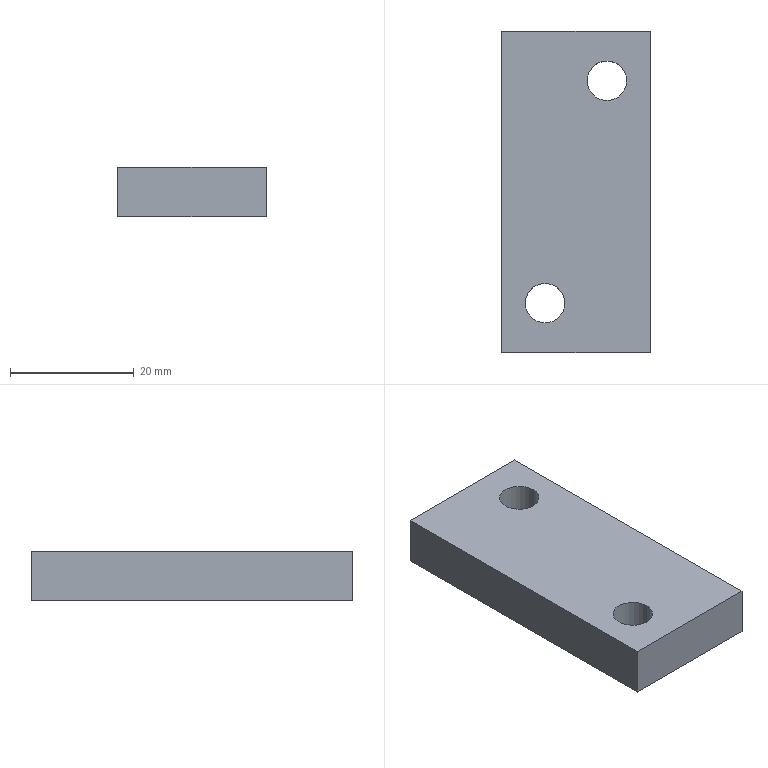Part | SolidWorks | features Extrusion 1, ICE 1 | 1 solid | 10 faces | box 24 x 52 x 8 mm | volume 9469 mm3 | plane 6 | cylinder 4 | commonest cylinder face diameters 6.4 x4
STEP:
#1=CARTESIAN_POINT('',(-8.2,-18.,-4.));
#2=VERTEX_POINT('',#1);
#3=CARTESIAN_POINT('',(-1.8,-18.,-4.));
#4=VERTEX_POINT('',#3);
#5=CARTESIAN_POINT('',(-5.,-18.,-4.));
#6=DIRECTION('',(0.,0.,1.));
#7=DIRECTION('',(1.,0.,0.));
#8=AXIS2_PLACEMENT_3D('',#5,#6,#7);
#9=CIRCLE('',#8,3.2);
#10=EDGE_CURVE('',#2,#4,#9,.T.);
#11=ORIENTED_EDGE('',*,*,#10,.F.);
#12=CARTESIAN_POINT('',(-8.2,-18.,4.));
#13=VERTEX_POINT('',#12);
#14=CARTESIAN_POINT('',(-8.2,-18.,-14.));
#15=DIRECTION('',(0.,0.,1.));
#16=VECTOR('',#15,1000.);
#17=LINE('',#14,#16);
#18=EDGE_CURVE('',#2,#13,#17,.T.);
#19=ORIENTED_EDGE('',*,*,#18,.T.);
#20=CARTESIAN_POINT('',(-1.8,-18.,4.));
#21=VERTEX_POINT('',#20);
#22=CARTESIAN_POINT('',(-5.,-18.,4.));
#23=DIRECTION('',(0.,0.,1.));
#24=DIRECTION('',(1.,0.,0.));
#25=AXIS2_PLACEMENT_3D('',#22,#23,#24);
#26=CIRCLE('',#25,3.2);
#27=EDGE_CURVE('',#13,#21,#26,.T.);
#28=ORIENTED_EDGE('',*,*,#27,.T.);
#29=CARTESIAN_POINT('',(-1.8,-18.,-14.));
#30=DIRECTION('',(0.,0.,1.));
#31=VECTOR('',#30,1000.);
#32=LINE('',#29,#31);
#33=EDGE_CURVE('',#4,#21,#32,.T.);
#34=ORIENTED_EDGE('',*,*,#33,.F.);
#35=EDGE_LOOP('',(#11,#19,#28,#34));
#36=FACE_OUTER_BOUND('',#35,.T.);
#37=CARTESIAN_POINT('',(-5.,-18.,-14.));
#38=DIRECTION('',(0.,0.,1.));
#39=DIRECTION('',(1.,0.,0.));
#40=AXIS2_PLACEMENT_3D('',#37,#38,#39);
#41=CYLINDRICAL_SURFACE('',#40,3.2);
#42=ADVANCED_FACE('',(#36),#41,.F.);
#43=CARTESIAN_POINT('',(1.8,18.,-4.));
#44=VERTEX_POINT('',#43);
#45=CARTESIAN_POINT('',(8.2,18.,-4.));
#46=VERTEX_POINT('',#45);
#47=CARTESIAN_POINT('',(5.,18.,-4.));
#48=DIRECTION('',(0.,0.,1.));
#49=DIRECTION('',(1.,0.,0.));
#50=AXIS2_PLACEMENT_3D('',#47,#48,#49);
#51=CIRCLE('',#50,3.2);
#52=EDGE_CURVE('',#44,#46,#51,.T.);
#53=ORIENTED_EDGE('',*,*,#52,.F.);
#54=CARTESIAN_POINT('',(1.8,18.,4.));
#55=VERTEX_POINT('',#54);
#56=CARTESIAN_POINT('',(1.8,18.,-14.));
#57=DIRECTION('',(0.,0.,1.));
#58=VECTOR('',#57,1000.);
#59=LINE('',#56,#58);
#60=EDGE_CURVE('',#44,#55,#59,.T.);
#61=ORIENTED_EDGE('',*,*,#60,.T.);
#62=CARTESIAN_POINT('',(8.2,18.,4.));
#63=VERTEX_POINT('',#62);
#64=CARTESIAN_POINT('',(5.,18.,4.));
#65=DIRECTION('',(0.,0.,1.));
#66=DIRECTION('',(1.,0.,0.));
#67=AXIS2_PLACEMENT_3D('',#64,#65,#66);
#68=CIRCLE('',#67,3.2);
#69=EDGE_CURVE('',#55,#63,#68,.T.);
#70=ORIENTED_EDGE('',*,*,#69,.T.);
#71=CARTESIAN_POINT('',(8.2,18.,-14.));
#72=DIRECTION('',(0.,0.,1.));
#73=VECTOR('',#72,1000.);
#74=LINE('',#71,#73);
#75=EDGE_CURVE('',#46,#63,#74,.T.);
#76=ORIENTED_EDGE('',*,*,#75,.F.);
#77=EDGE_LOOP('',(#53,#61,#70,#76));
#78=FACE_OUTER_BOUND('',#77,.T.);
#79=CARTESIAN_POINT('',(5.,18.,-14.));
#80=DIRECTION('',(0.,0.,1.));
#81=DIRECTION('',(1.,0.,0.));
#82=AXIS2_PLACEMENT_3D('',#79,#80,#81);
#83=CYLINDRICAL_SURFACE('',#82,3.2);
#84=ADVANCED_FACE('',(#78),#83,.F.);
#85=CARTESIAN_POINT('',(-12.,26.,4.));
#86=VERTEX_POINT('',#85);
#87=CARTESIAN_POINT('',(-12.,-26.,4.));
#88=VERTEX_POINT('',#87);
#89=CARTESIAN_POINT('',(-12.,26.,4.));
#90=DIRECTION('',(0.,-1.,0.));
#91=VECTOR('',#90,1000.);
#92=LINE('',#89,#91);
#93=EDGE_CURVE('',#86,#88,#92,.T.);
#94=ORIENTED_EDGE('',*,*,#93,.F.);
#95=CARTESIAN_POINT('',(-12.,26.,-4.));
#96=VERTEX_POINT('',#95);
#97=CARTESIAN_POINT('',(-12.,26.,-4.));
#98=DIRECTION('',(0.,0.,1.));
#99=VECTOR('',#98,1000.);
#100=LINE('',#97,#99);
#101=EDGE_CURVE('',#96,#86,#100,.T.);
#102=ORIENTED_EDGE('',*,*,#101,.F.);
#103=CARTESIAN_POINT('',(-12.,-26.,-4.));
#104=VERTEX_POINT('',#103);
#105=CARTESIAN_POINT('',(-12.,26.,-4.));
#106=DIRECTION('',(0.,-1.,0.));
#107=VECTOR('',#106,1000.);
#108=LINE('',#105,#107);
#109=EDGE_CURVE('',#96,#104,#108,.T.);
#110=ORIENTED_EDGE('',*,*,#109,.T.);
#111=CARTESIAN_POINT('',(-12.,-26.,-4.));
#112=DIRECTION('',(0.,0.,1.));
#113=VECTOR('',#112,1000.);
#114=LINE('',#111,#113);
#115=EDGE_CURVE('',#104,#88,#114,.T.);
#116=ORIENTED_EDGE('',*,*,#115,.T.);
#117=EDGE_LOOP('',(#94,#102,#110,#116));
#118=FACE_OUTER_BOUND('',#117,.T.);
#119=CARTESIAN_POINT('',(-12.,26.,-4.));
#120=DIRECTION('',(-1.,0.,0.));
#121=DIRECTION('',(0.,0.,1.));
#122=AXIS2_PLACEMENT_3D('',#119,#120,#121);
#123=PLANE('',#122);
#124=ADVANCED_FACE('',(#118),#123,.T.);
#125=CARTESIAN_POINT('',(12.,26.,4.));
#126=VERTEX_POINT('',#125);
#127=CARTESIAN_POINT('',(12.,26.,4.));
#128=DIRECTION('',(-1.,0.,0.));
#129=VECTOR('',#128,1000.);
#130=LINE('',#127,#129);
#131=EDGE_CURVE('',#126,#86,#130,.T.);
#132=ORIENTED_EDGE('',*,*,#131,.F.);
#133=CARTESIAN_POINT('',(12.,26.,-4.));
#134=VERTEX_POINT('',#133);
#135=CARTESIAN_POINT('',(12.,26.,-4.));
#136=DIRECTION('',(0.,0.,1.));
#137=VECTOR('',#136,1000.);
#138=LINE('',#135,#137);
#139=EDGE_CURVE('',#134,#126,#138,.T.);
#140=ORIENTED_EDGE('',*,*,#139,.F.);
#141=CARTESIAN_POINT('',(12.,26.,-4.));
#142=DIRECTION('',(-1.,0.,0.));
#143=VECTOR('',#142,1000.);
#144=LINE('',#141,#143);
#145=EDGE_CURVE('',#134,#96,#144,.T.);
#146=ORIENTED_EDGE('',*,*,#145,.T.);
#147=ORIENTED_EDGE('',*,*,#101,.T.);
#148=EDGE_LOOP('',(#132,#140,#146,#147));
#149=FACE_OUTER_BOUND('',#148,.T.);
#150=CARTESIAN_POINT('',(12.,26.,-4.));
#151=DIRECTION('',(0.,1.,0.));
#152=DIRECTION('',(0.,0.,1.));
#153=AXIS2_PLACEMENT_3D('',#150,#151,#152);
#154=PLANE('',#153);
#155=ADVANCED_FACE('',(#149),#154,.T.);
#156=CARTESIAN_POINT('',(12.,-26.,4.));
#157=VERTEX_POINT('',#156);
#158=CARTESIAN_POINT('',(12.,-26.,4.));
#159=DIRECTION('',(0.,1.,0.));
#160=VECTOR('',#159,1000.);
#161=LINE('',#158,#160);
#162=EDGE_CURVE('',#157,#126,#161,.T.);
#163=ORIENTED_EDGE('',*,*,#162,.F.);
#164=CARTESIAN_POINT('',(12.,-26.,-4.));
#165=VERTEX_POINT('',#164);
#166=CARTESIAN_POINT('',(12.,-26.,-4.));
#167=DIRECTION('',(0.,0.,1.));
#168=VECTOR('',#167,1000.);
#169=LINE('',#166,#168);
#170=EDGE_CURVE('',#165,#157,#169,.T.);
#171=ORIENTED_EDGE('',*,*,#170,.F.);
#172=CARTESIAN_POINT('',(12.,-26.,-4.));
#173=DIRECTION('',(0.,1.,0.));
#174=VECTOR('',#173,1000.);
#175=LINE('',#172,#174);
#176=EDGE_CURVE('',#165,#134,#175,.T.);
#177=ORIENTED_EDGE('',*,*,#176,.T.);
#178=ORIENTED_EDGE('',*,*,#139,.T.);
#179=EDGE_LOOP('',(#163,#171,#177,#178));
#180=FACE_OUTER_BOUND('',#179,.T.);
#181=CARTESIAN_POINT('',(12.,-26.,-4.));
#182=DIRECTION('',(1.,0.,0.));
#183=DIRECTION('',(0.,0.,-1.));
#184=AXIS2_PLACEMENT_3D('',#181,#182,#183);
#185=PLANE('',#184);
#186=ADVANCED_FACE('',(#180),#185,.T.);
#187=CARTESIAN_POINT('',(-12.,-26.,4.));
#188=DIRECTION('',(1.,0.,0.));
#189=VECTOR('',#188,1000.);
#190=LINE('',#187,#189);
#191=EDGE_CURVE('',#88,#157,#190,.T.);
#192=ORIENTED_EDGE('',*,*,#191,.F.);
#193=ORIENTED_EDGE('',*,*,#115,.F.);
#194=CARTESIAN_POINT('',(-12.,-26.,-4.));
#195=DIRECTION('',(1.,0.,0.));
#196=VECTOR('',#195,1000.);
#197=LINE('',#194,#196);
#198=EDGE_CURVE('',#104,#165,#197,.T.);
#199=ORIENTED_EDGE('',*,*,#198,.T.);
#200=ORIENTED_EDGE('',*,*,#170,.T.);
#201=EDGE_LOOP('',(#192,#193,#199,#200));
#202=FACE_OUTER_BOUND('',#201,.T.);
#203=CARTESIAN_POINT('',(-12.,-26.,-4.));
#204=DIRECTION('',(0.,-1.,0.));
#205=DIRECTION('',(0.,0.,-1.));
#206=AXIS2_PLACEMENT_3D('',#203,#204,#205);
#207=PLANE('',#206);
#208=ADVANCED_FACE('',(#202),#207,.T.);
#209=CARTESIAN_POINT('',(-5.,-18.,-4.));
#210=DIRECTION('',(0.,0.,1.));
#211=DIRECTION('',(1.,0.,0.));
#212=AXIS2_PLACEMENT_3D('',#209,#210,#211);
#213=CIRCLE('',#212,3.2);
#214=EDGE_CURVE('',#4,#2,#213,.T.);
#215=ORIENTED_EDGE('',*,*,#214,.T.);
#216=ORIENTED_EDGE('',*,*,#10,.T.);
#217=EDGE_LOOP('',(#215,#216));
#218=FACE_BOUND('',#217,.T.);
#219=CARTESIAN_POINT('',(5.,18.,-4.));
#220=DIRECTION('',(0.,0.,1.));
#221=DIRECTION('',(1.,0.,0.));
#222=AXIS2_PLACEMENT_3D('',#219,#220,#221);
#223=CIRCLE('',#222,3.2);
#224=EDGE_CURVE('',#46,#44,#223,.T.);
#225=ORIENTED_EDGE('',*,*,#224,.T.);
#226=ORIENTED_EDGE('',*,*,#52,.T.);
#227=EDGE_LOOP('',(#225,#226));
#228=FACE_BOUND('',#227,.T.);
#229=ORIENTED_EDGE('',*,*,#109,.F.);
#230=ORIENTED_EDGE('',*,*,#145,.F.);
#231=ORIENTED_EDGE('',*,*,#176,.F.);
#232=ORIENTED_EDGE('',*,*,#198,.F.);
#233=EDGE_LOOP('',(#229,#230,#231,#232));
#234=FACE_OUTER_BOUND('',#233,.T.);
#235=CARTESIAN_POINT('',(0.,0.,-4.));
#236=DIRECTION('',(0.,0.,1.));
#237=DIRECTION('',(1.,0.,0.));
#238=AXIS2_PLACEMENT_3D('',#235,#236,#237);
#239=PLANE('',#238);
#240=ADVANCED_FACE('',(#218,#228,#234),#239,.F.);
#241=CARTESIAN_POINT('',(-5.,-18.,4.));
#242=DIRECTION('',(0.,0.,1.));
#243=DIRECTION('',(1.,0.,0.));
#244=AXIS2_PLACEMENT_3D('',#241,#242,#243);
#245=CIRCLE('',#244,3.2);
#246=EDGE_CURVE('',#21,#13,#245,.T.);
#247=ORIENTED_EDGE('',*,*,#246,.F.);
#248=ORIENTED_EDGE('',*,*,#27,.F.);
#249=EDGE_LOOP('',(#247,#248));
#250=FACE_BOUND('',#249,.T.);
#251=CARTESIAN_POINT('',(5.,18.,4.));
#252=DIRECTION('',(0.,0.,1.));
#253=DIRECTION('',(1.,0.,0.));
#254=AXIS2_PLACEMENT_3D('',#251,#252,#253);
#255=CIRCLE('',#254,3.2);
#256=EDGE_CURVE('',#63,#55,#255,.T.);
#257=ORIENTED_EDGE('',*,*,#256,.F.);
#258=ORIENTED_EDGE('',*,*,#69,.F.);
#259=EDGE_LOOP('',(#257,#258));
#260=FACE_BOUND('',#259,.T.);
#261=ORIENTED_EDGE('',*,*,#93,.T.);
#262=ORIENTED_EDGE('',*,*,#191,.T.);
#263=ORIENTED_EDGE('',*,*,#162,.T.);
#264=ORIENTED_EDGE('',*,*,#131,.T.);
#265=EDGE_LOOP('',(#261,#262,#263,#264));
#266=FACE_OUTER_BOUND('',#265,.T.);
#267=CARTESIAN_POINT('',(0.,0.,4.));
#268=DIRECTION('',(0.,0.,1.));
#269=DIRECTION('',(1.,0.,0.));
#270=AXIS2_PLACEMENT_3D('',#267,#268,#269);
#271=PLANE('',#270);
#272=ADVANCED_FACE('',(#250,#260,#266),#271,.T.);
#273=ORIENTED_EDGE('',*,*,#60,.F.);
#274=ORIENTED_EDGE('',*,*,#224,.F.);
#275=ORIENTED_EDGE('',*,*,#75,.T.);
#276=ORIENTED_EDGE('',*,*,#256,.T.);
#277=EDGE_LOOP('',(#273,#274,#275,#276));
#278=FACE_OUTER_BOUND('',#277,.T.);
#279=CARTESIAN_POINT('',(5.,18.,-14.));
#280=DIRECTION('',(0.,0.,1.));
#281=DIRECTION('',(1.,0.,0.));
#282=AXIS2_PLACEMENT_3D('',#279,#280,#281);
#283=CYLINDRICAL_SURFACE('',#282,3.2);
#284=ADVANCED_FACE('',(#278),#283,.F.);
#285=ORIENTED_EDGE('',*,*,#18,.F.);
#286=ORIENTED_EDGE('',*,*,#214,.F.);
#287=ORIENTED_EDGE('',*,*,#33,.T.);
#288=ORIENTED_EDGE('',*,*,#246,.T.);
#289=EDGE_LOOP('',(#285,#286,#287,#288));
#290=FACE_OUTER_BOUND('',#289,.T.);
#291=CARTESIAN_POINT('',(-5.,-18.,-14.));
#292=DIRECTION('',(0.,0.,1.));
#293=DIRECTION('',(1.,0.,0.));
#294=AXIS2_PLACEMENT_3D('',#291,#292,#293);
#295=CYLINDRICAL_SURFACE('',#294,3.2);
#296=ADVANCED_FACE('',(#290),#295,.F.);
#297=CLOSED_SHELL('',(#42,#84,#124,#155,#186,#208,#240,#272,#284,#296));
#298=MANIFOLD_SOLID_BREP('',#297);
#299=CARTESIAN_POINT('',(0.,0.,0.));
#300=DIRECTION('',(0.,0.,1.));
#301=DIRECTION('',(1.,0.,0.));
#302=AXIS2_PLACEMENT_3D('',#299,#300,#301);
#303=(LENGTH_UNIT()NAMED_UNIT(*)SI_UNIT(.MILLI.,.METRE.));
#304=UNCERTAINTY_MEASURE_WITH_UNIT(LENGTH_MEASURE(0.00001),#303,'','');
#305=(NAMED_UNIT(*)PLANE_ANGLE_UNIT()SI_UNIT($,.RADIAN.));
#306=(NAMED_UNIT(*)SI_UNIT($,.STERADIAN.)SOLID_ANGLE_UNIT());
#307=(GEOMETRIC_REPRESENTATION_CONTEXT(3)GLOBAL_UNCERTAINTY_ASSIGNED_CONTEXT((#304))GLOBAL_UNIT_ASSIGNED_CONTEXT((#303,#305,#306))REPRESENTATION_CONTEXT('',''));
#308=ADVANCED_BREP_SHAPE_REPRESENTATION('',(#298,#302),#307);